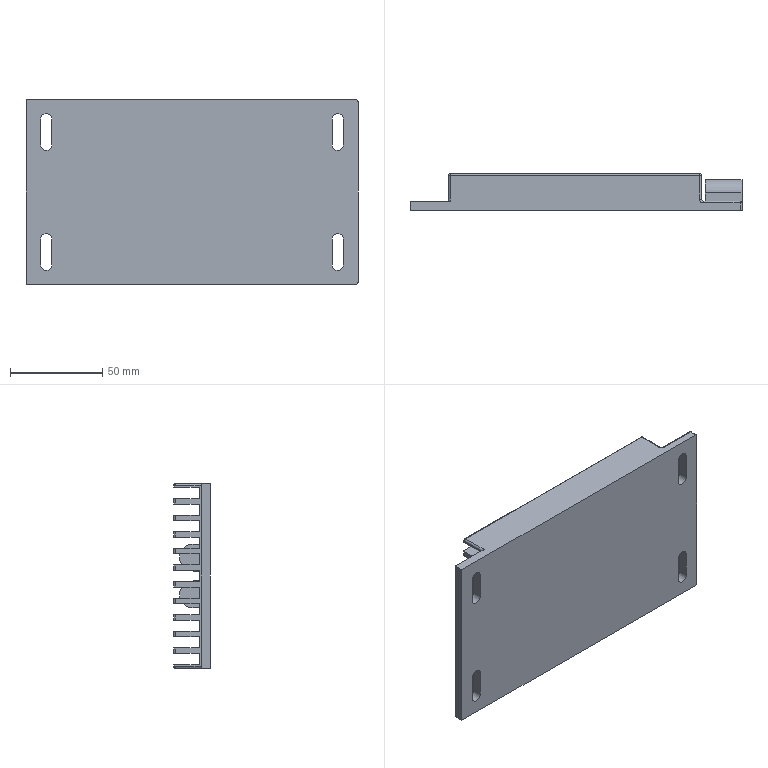Part | STEP file | Heater | 3 solids | 141 faces | box 180 x 20 x 100 mm | volume 172535 mm3 | plane 83 | cylinder 50 | sphere 6 | torus 2 | commonest cylinder face diameters 2 x36 6 x12 14.641 x2